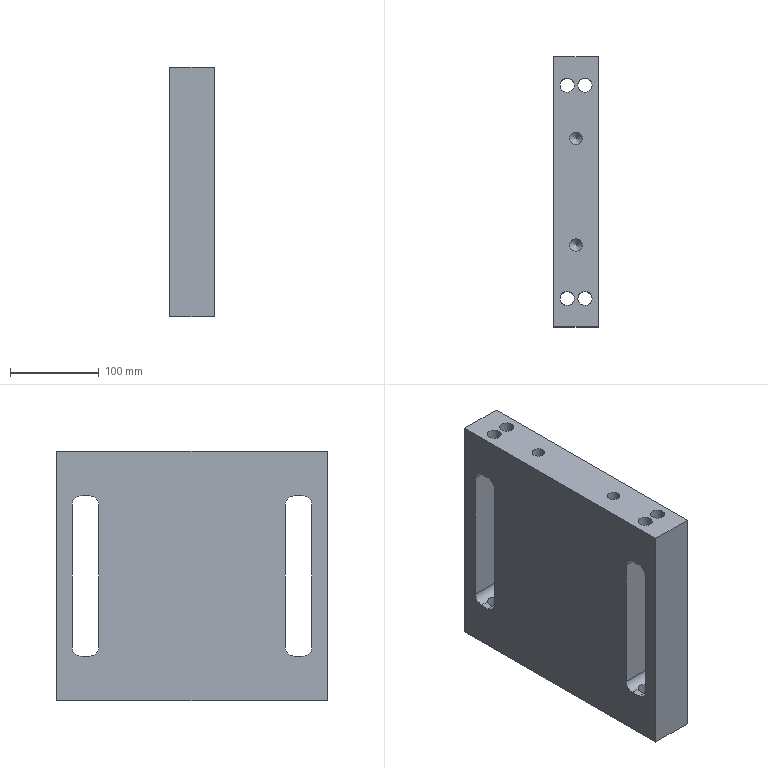Part | NX | features 29 2 | 1 solid | 46 faces | box 50 x 304 x 280.5 mm | volume 3625666 mm3 | plane 22 | cylinder 20 | cone 4 | commonest cylinder face diameters 16 x8 20 x8 14.1 x4